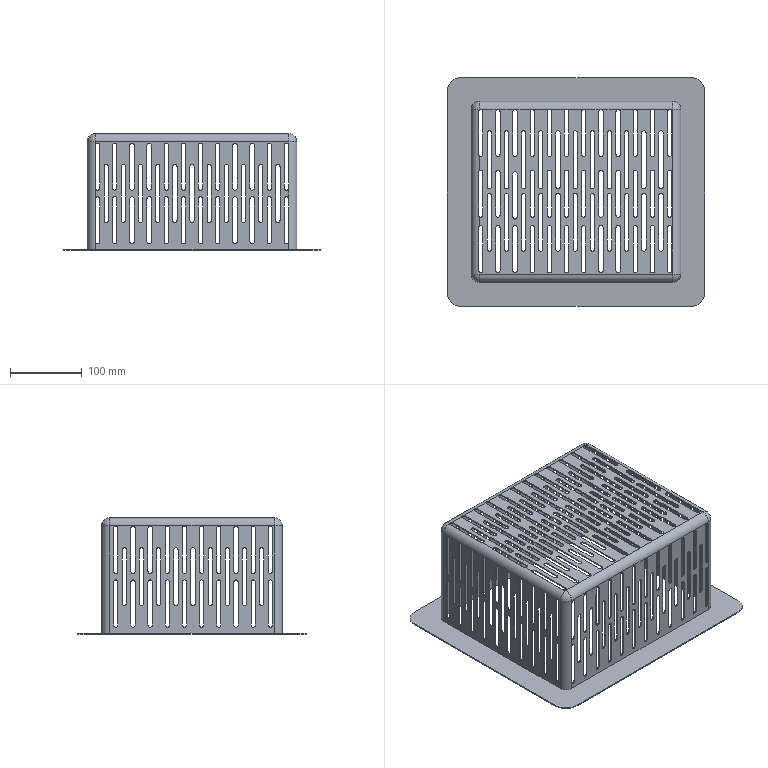Part | SolidWorks | features ICE 5, Fillet 3, Extrusion 1 | 1 solid | 860 faces | box 360 x 320 x 163 mm | volume 306732 mm3 | cylinder 462 | plane 390 | sphere 8 | commonest cylinder face diameters 6 x442 20 x8 23 x8 40 x4